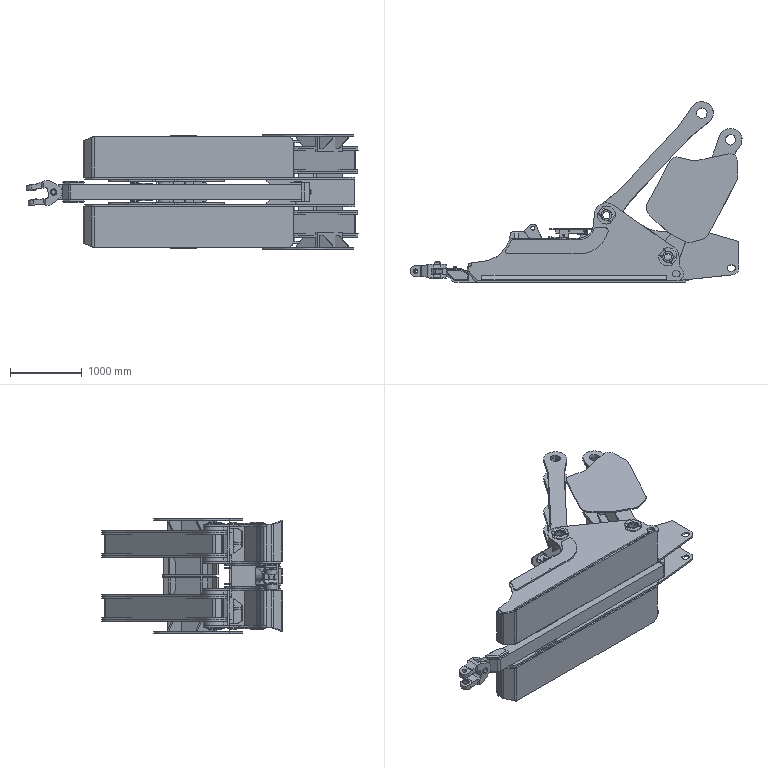Part | NX | features 底座(默认<按焊接>) 68, 前连杆 16, 后连杆右 14, 后连杆左 14, 推移千斤顶活塞 2, 推移千斤顶约束块 2, 推移千斤顶约束销 2, 推移千斤顶缸 2, 推移杆 2, 推移杆柱销 2, 推移杆连接头 2, 推移杆连接头销柱 2, 脚踏板 2, 脚踏板柱销 2 | 79 solids | 1772 faces | box 4616 x 2509 x 1594 mm | volume 1068302240 mm3 | plane 1216 | cylinder 532 | cone 13 | torus 7 | sphere 2 | spline 2 | commonest cylinder face diameters 200 x88 40 x46 100 x44 20 x41 60 x32 145 x30